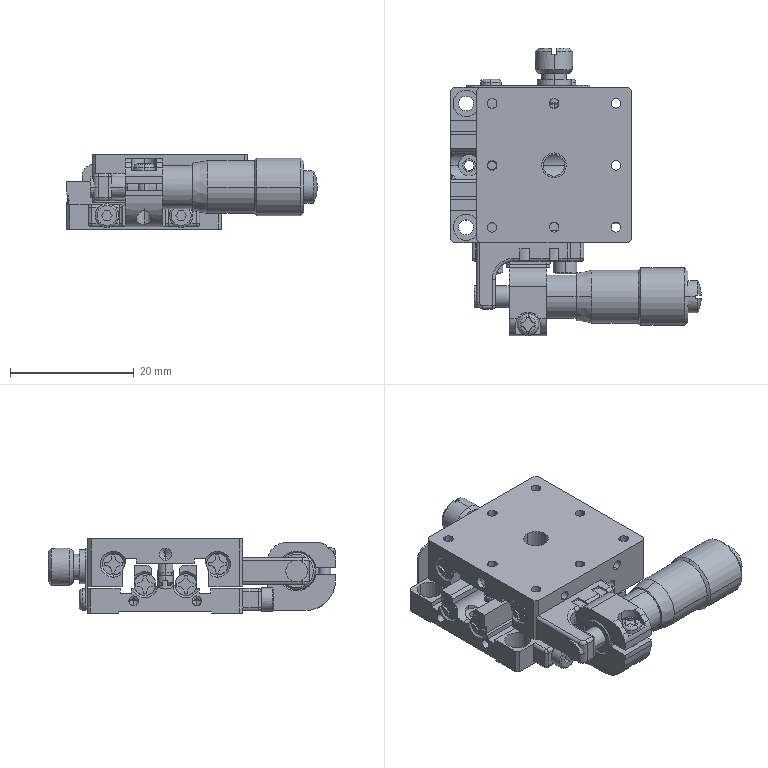Part | SolidWorks | 1 solid | 971 faces | box 40.495 x 46.4 x 12 mm | volume 8239 mm3 | plane 380 | cylinder 371 | cone 188 | torus 14 | sphere 14 | spline 4 | commonest cylinder face diameters 1.567 x70 2 x69 1.6 x38 1 x33 3.5 x30 2.4 x24